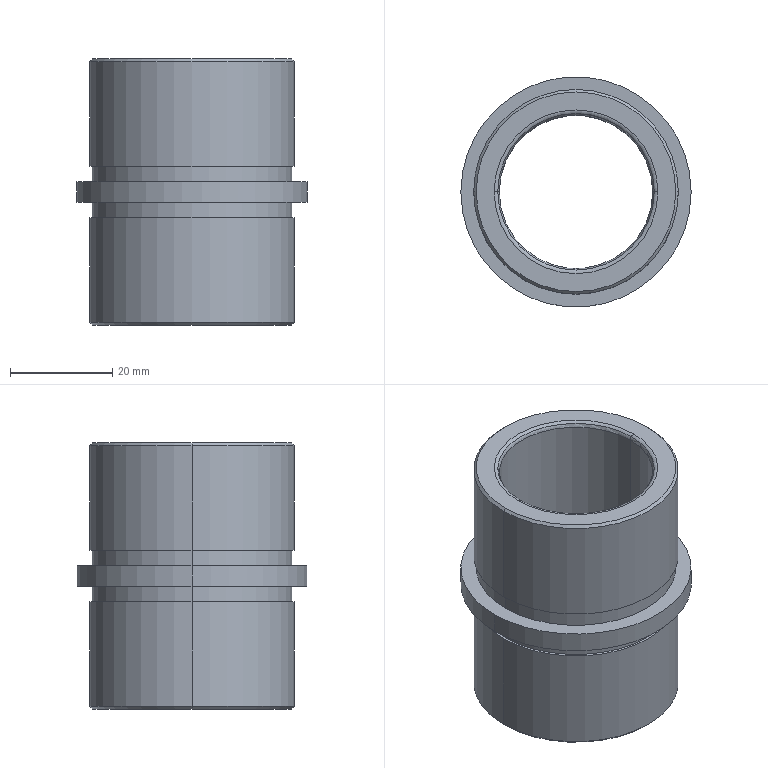Part | Creo | 1 solid | 30 faces | box 45 x 45 x 52 mm | volume 29479 mm3 | cylinder 12 | torus 8 | plane 6 | cone 4 | commonest cylinder face diameters 39 x4 40 x4 30 x2 45 x2
STEP:
#1=CARTESIAN_POINT('',(-187.5,-320.,-239.5));
#2=VERTEX_POINT('',#1);
#3=CARTESIAN_POINT('',(-142.5,-320.,-239.5));
#4=VERTEX_POINT('',#3);
#5=CARTESIAN_POINT('',(-165.,-320.,-239.5));
#6=DIRECTION('',(0.,0.,-1.));
#7=DIRECTION('',(-1.,0.,0.));
#8=AXIS2_PLACEMENT_3D('',#5,#6,#7);
#9=CIRCLE('',#8,22.5);
#10=EDGE_CURVE('',#2,#4,#9,.T.);
#11=ORIENTED_EDGE('',*,*,#10,.T.);
#12=CARTESIAN_POINT('',(-142.5,-320.,-235.5));
#13=VERTEX_POINT('',#12);
#14=CARTESIAN_POINT('',(-142.5,-320.,-239.5));
#15=DIRECTION('',(0.,0.,1.));
#16=VECTOR('',#15,4.);
#17=LINE('',#14,#16);
#18=EDGE_CURVE('',#4,#13,#17,.T.);
#19=ORIENTED_EDGE('',*,*,#18,.T.);
#20=CARTESIAN_POINT('',(-187.5,-320.,-235.5));
#21=VERTEX_POINT('',#20);
#22=CARTESIAN_POINT('',(-165.,-320.,-235.5));
#23=DIRECTION('',(0.,0.,1.));
#24=DIRECTION('',(1.,0.,0.));
#25=AXIS2_PLACEMENT_3D('',#22,#23,#24);
#26=CIRCLE('',#25,22.5);
#27=EDGE_CURVE('',#13,#21,#26,.T.);
#28=ORIENTED_EDGE('',*,*,#27,.T.);
#29=CARTESIAN_POINT('',(-187.5,-320.,-239.5));
#30=DIRECTION('',(0.,0.,1.));
#31=VECTOR('',#30,4.);
#32=LINE('',#29,#31);
#33=EDGE_CURVE('',#2,#21,#32,.T.);
#34=ORIENTED_EDGE('',*,*,#33,.F.);
#35=EDGE_LOOP('',(#11,#19,#28,#34));
#36=FACE_OUTER_BOUND('',#35,.F.);
#37=CARTESIAN_POINT('',(-165.,-320.,-239.5));
#38=DIRECTION('',(0.,0.,1.));
#39=DIRECTION('',(1.,0.,0.));
#40=AXIS2_PLACEMENT_3D('',#37,#38,#39);
#41=CYLINDRICAL_SURFACE('',#40,22.5);
#42=ADVANCED_FACE('',(#36),#41,.T.);
#43=CARTESIAN_POINT('',(-165.,-320.,-239.5));
#44=DIRECTION('',(0.,0.,-1.));
#45=DIRECTION('',(1.,0.,0.));
#46=AXIS2_PLACEMENT_3D('',#43,#44,#45);
#47=CIRCLE('',#46,22.5);
#48=EDGE_CURVE('',#4,#2,#47,.T.);
#49=ORIENTED_EDGE('',*,*,#48,.F.);
#50=ORIENTED_EDGE('',*,*,#10,.F.);
#51=EDGE_LOOP('',(#49,#50));
#52=FACE_OUTER_BOUND('',#51,.F.);
#53=CARTESIAN_POINT('',(-184.5,-320.,-239.5));
#54=VERTEX_POINT('',#53);
#55=CARTESIAN_POINT('',(-145.5,-320.,-239.5));
#56=VERTEX_POINT('',#55);
#57=CARTESIAN_POINT('',(-165.,-320.,-239.5));
#58=DIRECTION('',(0.,0.,1.));
#59=DIRECTION('',(-1.,0.,0.));
#60=AXIS2_PLACEMENT_3D('',#57,#58,#59);
#61=CIRCLE('',#60,19.5);
#62=EDGE_CURVE('',#54,#56,#61,.T.);
#63=ORIENTED_EDGE('',*,*,#62,.F.);
#64=CARTESIAN_POINT('',(-165.,-320.,-239.5));
#65=DIRECTION('',(0.,0.,1.));
#66=DIRECTION('',(1.,0.,0.));
#67=AXIS2_PLACEMENT_3D('',#64,#65,#66);
#68=CIRCLE('',#67,19.5);
#69=EDGE_CURVE('',#56,#54,#68,.T.);
#70=ORIENTED_EDGE('',*,*,#69,.F.);
#71=EDGE_LOOP('',(#63,#70));
#72=FACE_BOUND('',#71,.F.);
#73=CARTESIAN_POINT('',(-165.,-320.,-239.5));
#74=DIRECTION('',(0.,0.,1.));
#75=DIRECTION('',(1.,0.,0.));
#76=AXIS2_PLACEMENT_3D('',#73,#74,#75);
#77=PLANE('',#76);
#78=ADVANCED_FACE('',(#52,#72),#77,.F.);
#79=ORIENTED_EDGE('',*,*,#48,.T.);
#80=ORIENTED_EDGE('',*,*,#33,.T.);
#81=CARTESIAN_POINT('',(-165.,-320.,-235.5));
#82=DIRECTION('',(0.,0.,1.));
#83=DIRECTION('',(-1.,0.,0.));
#84=AXIS2_PLACEMENT_3D('',#81,#82,#83);
#85=CIRCLE('',#84,22.5);
#86=EDGE_CURVE('',#21,#13,#85,.T.);
#87=ORIENTED_EDGE('',*,*,#86,.T.);
#88=ORIENTED_EDGE('',*,*,#18,.F.);
#89=EDGE_LOOP('',(#79,#80,#87,#88));
#90=FACE_OUTER_BOUND('',#89,.F.);
#91=CARTESIAN_POINT('',(-165.,-320.,-239.5));
#92=DIRECTION('',(0.,0.,1.));
#93=DIRECTION('',(1.,0.,0.));
#94=AXIS2_PLACEMENT_3D('',#91,#92,#93);
#95=CYLINDRICAL_SURFACE('',#94,22.5);
#96=ADVANCED_FACE('',(#90),#95,.T.);
#97=ORIENTED_EDGE('',*,*,#27,.F.);
#98=ORIENTED_EDGE('',*,*,#86,.F.);
#99=EDGE_LOOP('',(#97,#98));
#100=FACE_OUTER_BOUND('',#99,.F.);
#101=CARTESIAN_POINT('',(-184.5,-320.,-235.5));
#102=VERTEX_POINT('',#101);
#103=CARTESIAN_POINT('',(-145.5,-320.,-235.5));
#104=VERTEX_POINT('',#103);
#105=CARTESIAN_POINT('',(-165.,-320.,-235.5));
#106=DIRECTION('',(0.,0.,-1.));
#107=DIRECTION('',(-1.,0.,0.));
#108=AXIS2_PLACEMENT_3D('',#105,#106,#107);
#109=CIRCLE('',#108,19.5);
#110=EDGE_CURVE('',#102,#104,#109,.T.);
#111=ORIENTED_EDGE('',*,*,#110,.F.);
#112=CARTESIAN_POINT('',(-165.,-320.,-235.5));
#113=DIRECTION('',(0.,0.,-1.));
#114=DIRECTION('',(1.,0.,0.));
#115=AXIS2_PLACEMENT_3D('',#112,#113,#114);
#116=CIRCLE('',#115,19.5);
#117=EDGE_CURVE('',#104,#102,#116,.T.);
#118=ORIENTED_EDGE('',*,*,#117,.F.);
#119=EDGE_LOOP('',(#111,#118));
#120=FACE_BOUND('',#119,.F.);
#121=CARTESIAN_POINT('',(-165.,-320.,-235.5));
#122=DIRECTION('',(0.,0.,1.));
#123=DIRECTION('',(1.,0.,0.));
#124=AXIS2_PLACEMENT_3D('',#121,#122,#123);
#125=PLANE('',#124);
#126=ADVANCED_FACE('',(#100,#120),#125,.T.);
#127=CARTESIAN_POINT('',(-145.5,-320.,-232.5));
#128=VERTEX_POINT('',#127);
#129=CARTESIAN_POINT('',(-184.5,-320.,-232.5));
#130=VERTEX_POINT('',#129);
#131=CARTESIAN_POINT('',(-165.,-320.,-232.5));
#132=DIRECTION('',(0.,0.,1.));
#133=DIRECTION('',(1.,0.,0.));
#134=AXIS2_PLACEMENT_3D('',#131,#132,#133);
#135=CIRCLE('',#134,19.5);
#136=EDGE_CURVE('',#128,#130,#135,.T.);
#137=ORIENTED_EDGE('',*,*,#136,.T.);
#138=CARTESIAN_POINT('',(-184.5,-320.,-232.5));
#139=DIRECTION('',(0.,0.,-1.));
#140=VECTOR('',#139,3.);
#141=LINE('',#138,#140);
#142=EDGE_CURVE('',#130,#102,#141,.T.);
#143=ORIENTED_EDGE('',*,*,#142,.T.);
#144=ORIENTED_EDGE('',*,*,#110,.T.);
#145=CARTESIAN_POINT('',(-145.5,-320.,-232.5));
#146=DIRECTION('',(0.,0.,-1.));
#147=VECTOR('',#146,3.);
#148=LINE('',#145,#147);
#149=EDGE_CURVE('',#128,#104,#148,.T.);
#150=ORIENTED_EDGE('',*,*,#149,.F.);
#151=EDGE_LOOP('',(#137,#143,#144,#150));
#152=FACE_OUTER_BOUND('',#151,.F.);
#153=CARTESIAN_POINT('',(-165.,-320.,-295.7));
#154=DIRECTION('',(0.,0.,-1.));
#155=DIRECTION('',(-1.,0.,0.));
#156=AXIS2_PLACEMENT_3D('',#153,#154,#155);
#157=CYLINDRICAL_SURFACE('',#156,19.5);
#158=ADVANCED_FACE('',(#152),#157,.T.);
#159=CARTESIAN_POINT('',(-145.,-320.,-232.5));
#160=VERTEX_POINT('',#159);
#161=CARTESIAN_POINT('',(-185.,-320.,-232.5));
#162=VERTEX_POINT('',#161);
#163=CARTESIAN_POINT('',(-165.,-320.,-232.5));
#164=DIRECTION('',(0.,0.,-1.));
#165=DIRECTION('',(1.,0.,0.));
#166=AXIS2_PLACEMENT_3D('',#163,#164,#165);
#167=CIRCLE('',#166,20.);
#168=EDGE_CURVE('',#160,#162,#167,.T.);
#169=ORIENTED_EDGE('',*,*,#168,.F.);
#170=CARTESIAN_POINT('',(-165.,-320.,-232.5));
#171=DIRECTION('',(0.,0.,-1.));
#172=DIRECTION('',(-1.,0.,0.));
#173=AXIS2_PLACEMENT_3D('',#170,#171,#172);
#174=CIRCLE('',#173,20.);
#175=EDGE_CURVE('',#162,#160,#174,.T.);
#176=ORIENTED_EDGE('',*,*,#175,.F.);
#177=EDGE_LOOP('',(#169,#176));
#178=FACE_OUTER_BOUND('',#177,.F.);
#179=CARTESIAN_POINT('',(-165.,-320.,-232.5));
#180=DIRECTION('',(0.,0.,1.));
#181=DIRECTION('',(-1.,0.,0.));
#182=AXIS2_PLACEMENT_3D('',#179,#180,#181);
#183=CIRCLE('',#182,19.5);
#184=EDGE_CURVE('',#130,#128,#183,.T.);
#185=ORIENTED_EDGE('',*,*,#184,.F.);
#186=ORIENTED_EDGE('',*,*,#136,.F.);
#187=EDGE_LOOP('',(#185,#186));
#188=FACE_BOUND('',#187,.F.);
#189=CARTESIAN_POINT('',(-110.,-320.,-232.5));
#190=DIRECTION('',(0.,0.,1.));
#191=DIRECTION('',(1.,0.,0.));
#192=AXIS2_PLACEMENT_3D('',#189,#190,#191);
#193=PLANE('',#192);
#194=ADVANCED_FACE('',(#178,#188),#193,.F.);
#195=CARTESIAN_POINT('',(-185.,-320.,-212.));
#196=VERTEX_POINT('',#195);
#197=CARTESIAN_POINT('',(-145.,-320.,-212.));
#198=VERTEX_POINT('',#197);
#199=CARTESIAN_POINT('',(-165.,-320.,-212.));
#200=DIRECTION('',(0.,0.,1.));
#201=DIRECTION('',(-1.,0.,0.));
#202=AXIS2_PLACEMENT_3D('',#199,#200,#201);
#203=CIRCLE('',#202,20.);
#204=EDGE_CURVE('',#196,#198,#203,.T.);
#205=ORIENTED_EDGE('',*,*,#204,.T.);
#206=CARTESIAN_POINT('',(-145.,-320.,-232.5));
#207=DIRECTION('',(0.,0.,1.));
#208=VECTOR('',#207,20.5);
#209=LINE('',#206,#208);
#210=EDGE_CURVE('',#160,#198,#209,.T.);
#211=ORIENTED_EDGE('',*,*,#210,.F.);
#212=ORIENTED_EDGE('',*,*,#168,.T.);
#213=CARTESIAN_POINT('',(-185.,-320.,-232.5));
#214=DIRECTION('',(0.,0.,1.));
#215=VECTOR('',#214,20.5);
#216=LINE('',#213,#215);
#217=EDGE_CURVE('',#162,#196,#216,.T.);
#218=ORIENTED_EDGE('',*,*,#217,.T.);
#219=EDGE_LOOP('',(#205,#211,#212,#218));
#220=FACE_OUTER_BOUND('',#219,.F.);
#221=CARTESIAN_POINT('',(-165.,-320.,-235.5));
#222=DIRECTION('',(0.,0.,1.));
#223=DIRECTION('',(1.,0.,0.));
#224=AXIS2_PLACEMENT_3D('',#221,#222,#223);
#225=CYLINDRICAL_SURFACE('',#224,20.);
#226=ADVANCED_FACE('',(#220),#225,.T.);
#227=ORIENTED_EDGE('',*,*,#204,.F.);
#228=CARTESIAN_POINT('',(-184.5,-320.,-211.5));
#229=VERTEX_POINT('',#228);
#230=CARTESIAN_POINT('',(-184.5,-320.,-211.5));
#231=DIRECTION('',(-0.7071,0.,-0.7071));
#232=VECTOR('',#231,0.7071);
#233=LINE('',#230,#232);
#234=EDGE_CURVE('',#229,#196,#233,.T.);
#235=ORIENTED_EDGE('',*,*,#234,.F.);
#236=CARTESIAN_POINT('',(-145.5,-320.,-211.5));
#237=VERTEX_POINT('',#236);
#238=CARTESIAN_POINT('',(-165.,-320.,-211.5));
#239=DIRECTION('',(0.,0.,1.));
#240=DIRECTION('',(-1.,0.,0.));
#241=AXIS2_PLACEMENT_3D('',#238,#239,#240);
#242=CIRCLE('',#241,19.5);
#243=EDGE_CURVE('',#229,#237,#242,.T.);
#244=ORIENTED_EDGE('',*,*,#243,.T.);
#245=CARTESIAN_POINT('',(-145.5,-320.,-211.5));
#246=DIRECTION('',(0.7071,0.,-0.7071));
#247=VECTOR('',#246,0.7071);
#248=LINE('',#245,#247);
#249=EDGE_CURVE('',#237,#198,#248,.T.);
#250=ORIENTED_EDGE('',*,*,#249,.T.);
#251=EDGE_LOOP('',(#227,#235,#244,#250));
#252=FACE_OUTER_BOUND('',#251,.F.);
#253=CARTESIAN_POINT('',(-165.,-320.,-211.75));
#254=DIRECTION('',(0.,0.,-1.));
#255=DIRECTION('',(-1.,0.,0.));
#256=AXIS2_PLACEMENT_3D('',#253,#254,#255);
#257=CONICAL_SURFACE('',#256,19.75,45.);
#258=ADVANCED_FACE('',(#252),#257,.T.);
#259=CARTESIAN_POINT('',(-165.,-320.,-212.));
#260=DIRECTION('',(0.,0.,1.));
#261=DIRECTION('',(1.,0.,0.));
#262=AXIS2_PLACEMENT_3D('',#259,#260,#261);
#263=CIRCLE('',#262,20.);
#264=EDGE_CURVE('',#198,#196,#263,.T.);
#265=ORIENTED_EDGE('',*,*,#264,.F.);
#266=ORIENTED_EDGE('',*,*,#249,.F.);
#267=CARTESIAN_POINT('',(-165.,-320.,-211.5));
#268=DIRECTION('',(0.,0.,1.));
#269=DIRECTION('',(1.,0.,0.));
#270=AXIS2_PLACEMENT_3D('',#267,#268,#269);
#271=CIRCLE('',#270,19.5);
#272=EDGE_CURVE('',#237,#229,#271,.T.);
#273=ORIENTED_EDGE('',*,*,#272,.T.);
#274=ORIENTED_EDGE('',*,*,#234,.T.);
#275=EDGE_LOOP('',(#265,#266,#273,#274));
#276=FACE_OUTER_BOUND('',#275,.F.);
#277=CARTESIAN_POINT('',(-165.,-320.,-211.75));
#278=DIRECTION('',(0.,0.,-1.));
#279=DIRECTION('',(-1.,0.,0.));
#280=AXIS2_PLACEMENT_3D('',#277,#278,#279);
#281=CONICAL_SURFACE('',#280,19.75,45.);
#282=ADVANCED_FACE('',(#276),#281,.T.);
#283=ORIENTED_EDGE('',*,*,#264,.T.);
#284=ORIENTED_EDGE('',*,*,#217,.F.);
#285=ORIENTED_EDGE('',*,*,#175,.T.);
#286=ORIENTED_EDGE('',*,*,#210,.T.);
#287=EDGE_LOOP('',(#283,#284,#285,#286));
#288=FACE_OUTER_BOUND('',#287,.F.);
#289=CARTESIAN_POINT('',(-165.,-320.,-235.5));
#290=DIRECTION('',(0.,0.,1.));
#291=DIRECTION('',(1.,0.,0.));
#292=AXIS2_PLACEMENT_3D('',#289,#290,#291);
#293=CYLINDRICAL_SURFACE('',#292,20.);
#294=ADVANCED_FACE('',(#288),#293,.T.);
#295=ORIENTED_EDGE('',*,*,#272,.F.);
#296=ORIENTED_EDGE('',*,*,#243,.F.);
#297=EDGE_LOOP('',(#295,#296));
#298=FACE_OUTER_BOUND('',#297,.F.);
#299=CARTESIAN_POINT('',(-149.,-320.,-211.5));
#300=VERTEX_POINT('',#299);
#301=CARTESIAN_POINT('',(-181.,-320.,-211.5));
#302=VERTEX_POINT('',#301);
#303=CARTESIAN_POINT('',(-165.,-320.,-211.5));
#304=DIRECTION('',(0.,0.,-1.));
#305=DIRECTION('',(1.,0.,0.));
#306=AXIS2_PLACEMENT_3D('',#303,#304,#305);
#307=CIRCLE('',#306,16.);
#308=EDGE_CURVE('',#300,#302,#307,.T.);
#309=ORIENTED_EDGE('',*,*,#308,.F.);
#310=CARTESIAN_POINT('',(-165.,-320.,-211.5));
#311=DIRECTION('',(0.,0.,-1.));
#312=DIRECTION('',(-1.,0.,0.));
#313=AXIS2_PLACEMENT_3D('',#310,#311,#312);
#314=CIRCLE('',#313,16.);
#315=EDGE_CURVE('',#302,#300,#314,.T.);
#316=ORIENTED_EDGE('',*,*,#315,.F.);
#317=EDGE_LOOP('',(#309,#316));
#318=FACE_BOUND('',#317,.F.);
#319=CARTESIAN_POINT('',(-165.,-320.,-211.5));
#320=DIRECTION('',(0.,0.,1.));
#321=DIRECTION('',(1.,0.,0.));
#322=AXIS2_PLACEMENT_3D('',#319,#320,#321);
#323=PLANE('',#322);
#324=ADVANCED_FACE('',(#298,#318),#323,.T.);
#325=ORIENTED_EDGE('',*,*,#308,.T.);
#326=CARTESIAN_POINT('',(-180.293,-320.,-211.793));
#327=VERTEX_POINT('',#326);
#328=CARTESIAN_POINT('',(-181.,-320.,-212.5));
#329=DIRECTION('',(0.,1.,0.));
#330=DIRECTION('',(0.,0.,1.));
#331=AXIS2_PLACEMENT_3D('',#328,#329,#330);
#332=CIRCLE('',#331,1.);
#333=EDGE_CURVE('',#302,#327,#332,.T.);
#334=ORIENTED_EDGE('',*,*,#333,.T.);
#335=CARTESIAN_POINT('',(-149.707,-320.,-211.793));
#336=VERTEX_POINT('',#335);
#337=CARTESIAN_POINT('',(-165.,-320.,-211.793));
#338=DIRECTION('',(0.,0.,1.));
#339=DIRECTION('',(-1.,0.,0.));
#340=AXIS2_PLACEMENT_3D('',#337,#338,#339);
#341=CIRCLE('',#340,15.293);
#342=EDGE_CURVE('',#327,#336,#341,.T.);
#343=ORIENTED_EDGE('',*,*,#342,.T.);
#344=CARTESIAN_POINT('',(-149.,-320.,-212.5));
#345=DIRECTION('',(0.,-1.,0.));
#346=DIRECTION('',(0.,0.,1.));
#347=AXIS2_PLACEMENT_3D('',#344,#345,#346);
#348=CIRCLE('',#347,1.);
#349=EDGE_CURVE('',#300,#336,#348,.T.);
#350=ORIENTED_EDGE('',*,*,#349,.F.);
#351=EDGE_LOOP('',(#325,#334,#343,#350));
#352=FACE_OUTER_BOUND('',#351,.F.);
#353=CARTESIAN_POINT('',(-165.,-320.,-212.5));
#354=DIRECTION('',(0.,0.,1.));
#355=DIRECTION('',(1.,0.,0.));
#356=AXIS2_PLACEMENT_3D('',#353,#354,#355);
#357=TOROIDAL_SURFACE('',#356,16.,1.);
#358=ADVANCED_FACE('',(#352),#357,.T.);
#359=ORIENTED_EDGE('',*,*,#315,.T.);
#360=ORIENTED_EDGE('',*,*,#349,.T.);
#361=CARTESIAN_POINT('',(-165.,-320.,-211.793));
#362=DIRECTION('',(0.,0.,1.));
#363=DIRECTION('',(1.,0.,0.));
#364=AXIS2_PLACEMENT_3D('',#361,#362,#363);
#365=CIRCLE('',#364,15.293);
#366=EDGE_CURVE('',#336,#327,#365,.T.);
#367=ORIENTED_EDGE('',*,*,#366,.T.);
#368=ORIENTED_EDGE('',*,*,#333,.F.);
#369=EDGE_LOOP('',(#359,#360,#367,#368));
#370=FACE_OUTER_BOUND('',#369,.F.);
#371=CARTESIAN_POINT('',(-165.,-320.,-212.5));
#372=DIRECTION('',(0.,0.,1.));
#373=DIRECTION('',(1.,0.,0.));
#374=AXIS2_PLACEMENT_3D('',#371,#372,#373);
#375=TOROIDAL_SURFACE('',#374,16.,1.);
#376=ADVANCED_FACE('',(#370),#375,.T.);
#377=CARTESIAN_POINT('',(-180.,-320.,-212.5));
#378=VERTEX_POINT('',#377);
#379=CARTESIAN_POINT('',(-150.,-320.,-212.5));
#380=VERTEX_POINT('',#379);
#381=CARTESIAN_POINT('',(-165.,-320.,-212.5));
#382=DIRECTION('',(0.,0.,-1.));
#383=DIRECTION('',(-1.,0.,0.));
#384=AXIS2_PLACEMENT_3D('',#381,#382,#383);
#385=CIRCLE('',#384,15.);
#386=EDGE_CURVE('',#378,#380,#385,.T.);
#387=ORIENTED_EDGE('',*,*,#386,.F.);
#388=CARTESIAN_POINT('',(-181.,-320.,-212.5));
#389=DIRECTION('',(0.,1.,0.));
#390=DIRECTION('',(0.7071,0.,0.7071));
#391=AXIS2_PLACEMENT_3D('',#388,#389,#390);
#392=CIRCLE('',#391,1.);
#393=EDGE_CURVE('',#327,#378,#392,.T.);
#394=ORIENTED_EDGE('',*,*,#393,.F.);
#395=ORIENTED_EDGE('',*,*,#366,.F.);
#396=CARTESIAN_POINT('',(-149.,-320.,-212.5));
#397=DIRECTION('',(0.,-1.,0.));
#398=DIRECTION('',(-0.7071,0.,0.7071));
#399=AXIS2_PLACEMENT_3D('',#396,#397,#398);
#400=CIRCLE('',#399,1.);
#401=EDGE_CURVE('',#336,#380,#400,.T.);
#402=ORIENTED_EDGE('',*,*,#401,.T.);
#403=EDGE_LOOP('',(#387,#394,#395,#402));
#404=FACE_OUTER_BOUND('',#403,.F.);
#405=CARTESIAN_POINT('',(-165.,-320.,-212.5));
#406=DIRECTION('',(0.,0.,1.));
#407=DIRECTION('',(1.,0.,0.));
#408=AXIS2_PLACEMENT_3D('',#405,#406,#407);
#409=TOROIDAL_SURFACE('',#408,16.,1.);
#410=ADVANCED_FACE('',(#404),#409,.T.);
#411=CARTESIAN_POINT('',(-150.,-320.,-262.5));
#412=VERTEX_POINT('',#411);
#413=CARTESIAN_POINT('',(-180.,-320.,-262.5));
#414=VERTEX_POINT('',#413);
#415=CARTESIAN_POINT('',(-165.,-320.,-262.5));
#416=DIRECTION('',(0.,0.,1.));
#417=DIRECTION('',(1.,0.,0.));
#418=AXIS2_PLACEMENT_3D('',#415,#416,#417);
#419=CIRCLE('',#418,15.);
#420=EDGE_CURVE('',#412,#414,#419,.T.);
#421=ORIENTED_EDGE('',*,*,#420,.T.);
#422=CARTESIAN_POINT('',(-180.,-320.,-212.5));
#423=DIRECTION('',(0.,0.,-1.));
#424=VECTOR('',#423,50.);
#425=LINE('',#422,#424);
#426=EDGE_CURVE('',#378,#414,#425,.T.);
#427=ORIENTED_EDGE('',*,*,#426,.F.);
#428=ORIENTED_EDGE('',*,*,#386,.T.);
#429=CARTESIAN_POINT('',(-150.,-320.,-212.5));
#430=DIRECTION('',(0.,0.,-1.));
#431=VECTOR('',#430,50.);
#432=LINE('',#429,#431);
#433=EDGE_CURVE('',#380,#412,#432,.T.);
#434=ORIENTED_EDGE('',*,*,#433,.T.);
#435=EDGE_LOOP('',(#421,#427,#428,#434));
#436=FACE_OUTER_BOUND('',#435,.F.);
#437=CARTESIAN_POINT('',(-165.,-320.,-211.5));
#438=DIRECTION('',(0.,0.,-1.));
#439=DIRECTION('',(-1.,0.,0.));
#440=AXIS2_PLACEMENT_3D('',#437,#438,#439);
#441=CYLINDRICAL_SURFACE('',#440,15.);
#442=ADVANCED_FACE('',(#436),#441,.F.);
#443=ORIENTED_EDGE('',*,*,#420,.F.);
#444=CARTESIAN_POINT('',(-149.707,-320.,-263.207));
#445=VERTEX_POINT('',#444);
#446=CARTESIAN_POINT('',(-149.,-320.,-262.5));
#447=DIRECTION('',(0.,1.,0.));
#448=DIRECTION('',(-0.7071,0.,-0.7071));
#449=AXIS2_PLACEMENT_3D('',#446,#447,#448);
#450=CIRCLE('',#449,1.);
#451=EDGE_CURVE('',#445,#412,#450,.T.);
#452=ORIENTED_EDGE('',*,*,#451,.F.);
#453=CARTESIAN_POINT('',(-180.293,-320.,-263.207));
#454=VERTEX_POINT('',#453);
#455=CARTESIAN_POINT('',(-165.,-320.,-263.207));
#456=DIRECTION('',(0.,0.,-1.));
#457=DIRECTION('',(-1.,0.,0.));
#458=AXIS2_PLACEMENT_3D('',#455,#456,#457);
#459=CIRCLE('',#458,15.293);
#460=EDGE_CURVE('',#454,#445,#459,.T.);
#461=ORIENTED_EDGE('',*,*,#460,.F.);
#462=CARTESIAN_POINT('',(-181.,-320.,-262.5));
#463=DIRECTION('',(0.,-1.,0.));
#464=DIRECTION('',(0.7071,0.,-0.7071));
#465=AXIS2_PLACEMENT_3D('',#462,#463,#464);
#466=CIRCLE('',#465,1.);
#467=EDGE_CURVE('',#454,#414,#466,.T.);
#468=ORIENTED_EDGE('',*,*,#467,.T.);
#469=EDGE_LOOP('',(#443,#452,#461,#468));
#470=FACE_OUTER_BOUND('',#469,.F.);
#471=CARTESIAN_POINT('',(-165.,-320.,-262.5));
#472=DIRECTION('',(0.,0.,-1.));
#473=DIRECTION('',(-1.,0.,0.));
#474=AXIS2_PLACEMENT_3D('',#471,#472,#473);
#475=TOROIDAL_SURFACE('',#474,16.,1.);
#476=ADVANCED_FACE('',(#470),#475,.T.);
#477=CARTESIAN_POINT('',(-165.,-320.,-262.5));
#478=DIRECTION('',(0.,0.,1.));
#479=DIRECTION('',(-1.,0.,0.));
#480=AXIS2_PLACEMENT_3D('',#477,#478,#479);
#481=CIRCLE('',#480,15.);
#482=EDGE_CURVE('',#414,#412,#481,.T.);
#483=ORIENTED_EDGE('',*,*,#482,.F.);
#484=ORIENTED_EDGE('',*,*,#467,.F.);
#485=CARTESIAN_POINT('',(-165.,-320.,-263.207));
#486=DIRECTION('',(0.,0.,-1.));
#487=DIRECTION('',(1.,0.,0.));
#488=AXIS2_PLACEMENT_3D('',#485,#486,#487);
#489=CIRCLE('',#488,15.293);
#490=EDGE_CURVE('',#445,#454,#489,.T.);
#491=ORIENTED_EDGE('',*,*,#490,.F.);
#492=ORIENTED_EDGE('',*,*,#451,.T.);
#493=EDGE_LOOP('',(#483,#484,#491,#492));
#494=FACE_OUTER_BOUND('',#493,.F.);
#495=CARTESIAN_POINT('',(-165.,-320.,-262.5));
#496=DIRECTION('',(0.,0.,-1.));
#497=DIRECTION('',(-1.,0.,0.));
#498=AXIS2_PLACEMENT_3D('',#495,#496,#497);
#499=TOROIDAL_SURFACE('',#498,16.,1.);
#500=ADVANCED_FACE('',(#494),#499,.T.);
#501=ORIENTED_EDGE('',*,*,#482,.T.);
#502=ORIENTED_EDGE('',*,*,#433,.F.);
#503=CARTESIAN_POINT('',(-165.,-320.,-212.5));
#504=DIRECTION('',(0.,0.,-1.));
#505=DIRECTION('',(1.,0.,0.));
#506=AXIS2_PLACEMENT_3D('',#503,#504,#505);
#507=CIRCLE('',#506,15.);
#508=EDGE_CURVE('',#380,#378,#507,.T.);
#509=ORIENTED_EDGE('',*,*,#508,.T.);
#510=ORIENTED_EDGE('',*,*,#426,.T.);
#511=EDGE_LOOP('',(#501,#502,#509,#510));
#512=FACE_OUTER_BOUND('',#511,.F.);
#513=CARTESIAN_POINT('',(-165.,-320.,-211.5));
#514=DIRECTION('',(0.,0.,-1.));
#515=DIRECTION('',(-1.,0.,0.));
#516=AXIS2_PLACEMENT_3D('',#513,#514,#515);
#517=CYLINDRICAL_SURFACE('',#516,15.);
#518=ADVANCED_FACE('',(#512),#517,.F.);
#519=ORIENTED_EDGE('',*,*,#508,.F.);
#520=ORIENTED_EDGE('',*,*,#401,.F.);
#521=ORIENTED_EDGE('',*,*,#342,.F.);
#522=ORIENTED_EDGE('',*,*,#393,.T.);
#523=EDGE_LOOP('',(#519,#520,#521,#522));
#524=FACE_OUTER_BOUND('',#523,.F.);
#525=CARTESIAN_POINT('',(-165.,-320.,-212.5));
#526=DIRECTION('',(0.,0.,1.));
#527=DIRECTION('',(1.,0.,0.));
#528=AXIS2_PLACEMENT_3D('',#525,#526,#527);
#529=TOROIDAL_SURFACE('',#528,16.,1.);
#530=ADVANCED_FACE('',(#524),#529,.T.);
#531=CARTESIAN_POINT('',(-181.,-320.,-263.5));
#532=VERTEX_POINT('',#531);
#533=CARTESIAN_POINT('',(-149.,-320.,-263.5));
#534=VERTEX_POINT('',#533);
#535=CARTESIAN_POINT('',(-165.,-320.,-263.5));
#536=DIRECTION('',(0.,0.,1.));
#537=DIRECTION('',(-1.,0.,0.));
#538=AXIS2_PLACEMENT_3D('',#535,#536,#537);
#539=CIRCLE('',#538,16.);
#540=EDGE_CURVE('',#532,#534,#539,.T.);
#541=ORIENTED_EDGE('',*,*,#540,.T.);
#542=CARTESIAN_POINT('',(-149.,-320.,-262.5));
#543=DIRECTION('',(0.,1.,0.));
#544=DIRECTION('',(0.,0.,-1.));
#545=AXIS2_PLACEMENT_3D('',#542,#543,#544);
#546=CIRCLE('',#545,1.);
#547=EDGE_CURVE('',#534,#445,#546,.T.);
#548=ORIENTED_EDGE('',*,*,#547,.T.);
#549=ORIENTED_EDGE('',*,*,#490,.T.);
#550=CARTESIAN_POINT('',(-181.,-320.,-262.5));
#551=DIRECTION('',(0.,-1.,0.));
#552=DIRECTION('',(0.,0.,-1.));
#553=AXIS2_PLACEMENT_3D('',#550,#551,#552);
#554=CIRCLE('',#553,1.);
#555=EDGE_CURVE('',#532,#454,#554,.T.);
#556=ORIENTED_EDGE('',*,*,#555,.F.);
#557=EDGE_LOOP('',(#541,#548,#549,#556));
#558=FACE_OUTER_BOUND('',#557,.F.);
#559=CARTESIAN_POINT('',(-165.,-320.,-262.5));
#560=DIRECTION('',(0.,0.,-1.));
#561=DIRECTION('',(-1.,0.,0.));
#562=AXIS2_PLACEMENT_3D('',#559,#560,#561);
#563=TOROIDAL_SURFACE('',#562,16.,1.);
#564=ADVANCED_FACE('',(#558),#563,.T.);
#565=CARTESIAN_POINT('',(-184.5,-320.,-263.5));
#566=VERTEX_POINT('',#565);
#567=CARTESIAN_POINT('',(-145.5,-320.,-263.5));
#568=VERTEX_POINT('',#567);
#569=CARTESIAN_POINT('',(-165.,-320.,-263.5));
#570=DIRECTION('',(0.,0.,-1.));
#571=DIRECTION('',(-1.,0.,0.));
#572=AXIS2_PLACEMENT_3D('',#569,#570,#571);
#573=CIRCLE('',#572,19.5);
#574=EDGE_CURVE('',#566,#568,#573,.T.);
#575=ORIENTED_EDGE('',*,*,#574,.F.);
#576=CARTESIAN_POINT('',(-165.,-320.,-263.5));
#577=DIRECTION('',(0.,0.,-1.));
#578=DIRECTION('',(1.,0.,0.));
#579=AXIS2_PLACEMENT_3D('',#576,#577,#578);
#580=CIRCLE('',#579,19.5);
#581=EDGE_CURVE('',#568,#566,#580,.T.);
#582=ORIENTED_EDGE('',*,*,#581,.F.);
#583=EDGE_LOOP('',(#575,#582));
#584=FACE_OUTER_BOUND('',#583,.F.);
#585=ORIENTED_EDGE('',*,*,#540,.F.);
#586=CARTESIAN_POINT('',(-165.,-320.,-263.5));
#587=DIRECTION('',(0.,0.,1.));
#588=DIRECTION('',(1.,0.,0.));
#589=AXIS2_PLACEMENT_3D('',#586,#587,#588);
#590=CIRCLE('',#589,16.);
#591=EDGE_CURVE('',#534,#532,#590,.T.);
#592=ORIENTED_EDGE('',*,*,#591,.F.);
#593=EDGE_LOOP('',(#585,#592));
#594=FACE_BOUND('',#593,.F.);
#595=CARTESIAN_POINT('',(-165.,-320.,-263.5));
#596=DIRECTION('',(0.,0.,-1.));
#597=DIRECTION('',(-1.,0.,0.));
#598=AXIS2_PLACEMENT_3D('',#595,#596,#597);
#599=PLANE('',#598);
#600=ADVANCED_FACE('',(#584,#594),#599,.T.);
#601=CARTESIAN_POINT('',(-185.,-320.,-263.));
#602=VERTEX_POINT('',#601);
#603=CARTESIAN_POINT('',(-145.,-320.,-263.));
#604=VERTEX_POINT('',#603);
#605=CARTESIAN_POINT('',(-165.,-320.,-263.));
#606=DIRECTION('',(0.,0.,-1.));
#607=DIRECTION('',(-1.,0.,0.));
#608=AXIS2_PLACEMENT_3D('',#605,#606,#607);
#609=CIRCLE('',#608,20.);
#610=EDGE_CURVE('',#602,#604,#609,.T.);
#611=ORIENTED_EDGE('',*,*,#610,.F.);
#612=CARTESIAN_POINT('',(-184.5,-320.,-263.5));
#613=DIRECTION('',(-0.7071,0.,0.7071));
#614=VECTOR('',#613,0.7071);
#615=LINE('',#612,#614);
#616=EDGE_CURVE('',#566,#602,#615,.T.);
#617=ORIENTED_EDGE('',*,*,#616,.F.);
#618=ORIENTED_EDGE('',*,*,#574,.T.);
#619=CARTESIAN_POINT('',(-145.5,-320.,-263.5));
#620=DIRECTION('',(0.7071,0.,0.7071));
#621=VECTOR('',#620,0.7071);
#622=LINE('',#619,#621);
#623=EDGE_CURVE('',#568,#604,#622,.T.);
#624=ORIENTED_EDGE('',*,*,#623,.T.);
#625=EDGE_LOOP('',(#611,#617,#618,#624));
#626=FACE_OUTER_BOUND('',#625,.F.);
#627=CARTESIAN_POINT('',(-165.,-320.,-263.25));
#628=DIRECTION('',(0.,0.,1.));
#629=DIRECTION('',(1.,0.,0.));
#630=AXIS2_PLACEMENT_3D('',#627,#628,#629);
#631=CONICAL_SURFACE('',#630,19.75,45.);
#632=ADVANCED_FACE('',(#626),#631,.T.);
#633=ORIENTED_EDGE('',*,*,#610,.T.);
#634=CARTESIAN_POINT('',(-145.,-320.,-242.5));
#635=VERTEX_POINT('',#634);
#636=CARTESIAN_POINT('',(-145.,-320.,-242.5));
#637=DIRECTION('',(0.,0.,-1.));
#638=VECTOR('',#637,20.5);
#639=LINE('',#636,#638);
#640=EDGE_CURVE('',#635,#604,#639,.T.);
#641=ORIENTED_EDGE('',*,*,#640,.F.);
#642=CARTESIAN_POINT('',(-185.,-320.,-242.5));
#643=VERTEX_POINT('',#642);
#644=CARTESIAN_POINT('',(-165.,-320.,-242.5));
#645=DIRECTION('',(0.,0.,1.));
#646=DIRECTION('',(1.,0.,0.));
#647=AXIS2_PLACEMENT_3D('',#644,#645,#646);
#648=CIRCLE('',#647,20.);
#649=EDGE_CURVE('',#635,#643,#648,.T.);
#650=ORIENTED_EDGE('',*,*,#649,.T.);
#651=CARTESIAN_POINT('',(-185.,-320.,-242.5));
#652=DIRECTION('',(0.,0.,-1.));
#653=VECTOR('',#652,20.5);
#654=LINE('',#651,#653);
#655=EDGE_CURVE('',#643,#602,#654,.T.);
#656=ORIENTED_EDGE('',*,*,#655,.T.);
#657=EDGE_LOOP('',(#633,#641,#650,#656));
#658=FACE_OUTER_BOUND('',#657,.F.);
#659=CARTESIAN_POINT('',(-165.,-320.,-239.5));
#660=DIRECTION('',(0.,0.,-1.));
#661=DIRECTION('',(-1.,0.,0.));
#662=AXIS2_PLACEMENT_3D('',#659,#660,#661);
#663=CYLINDRICAL_SURFACE('',#662,20.);
#664=ADVANCED_FACE('',(#658),#663,.T.);
#665=CARTESIAN_POINT('',(-165.,-320.,-263.));
#666=DIRECTION('',(0.,0.,-1.));
#667=DIRECTION('',(1.,0.,0.));
#668=AXIS2_PLACEMENT_3D('',#665,#666,#667);
#669=CIRCLE('',#668,20.);
#670=EDGE_CURVE('',#604,#602,#669,.T.);
#671=ORIENTED_EDGE('',*,*,#670,.T.);
#672=ORIENTED_EDGE('',*,*,#655,.F.);
#673=CARTESIAN_POINT('',(-165.,-320.,-242.5));
#674=DIRECTION('',(0.,0.,1.));
#675=DIRECTION('',(-1.,0.,0.));
#676=AXIS2_PLACEMENT_3D('',#673,#674,#675);
#677=CIRCLE('',#676,20.);
#678=EDGE_CURVE('',#643,#635,#677,.T.);
#679=ORIENTED_EDGE('',*,*,#678,.T.);
#680=ORIENTED_EDGE('',*,*,#640,.T.);
#681=EDGE_LOOP('',(#671,#672,#679,#680));
#682=FACE_OUTER_BOUND('',#681,.F.);
#683=CARTESIAN_POINT('',(-165.,-320.,-239.5));
#684=DIRECTION('',(0.,0.,-1.));
#685=DIRECTION('',(-1.,0.,0.));
#686=AXIS2_PLACEMENT_3D('',#683,#684,#685);
#687=CYLINDRICAL_SURFACE('',#686,20.);
#688=ADVANCED_FACE('',(#682),#687,.T.);
#689=ORIENTED_EDGE('',*,*,#670,.F.);
#690=ORIENTED_EDGE('',*,*,#623,.F.);
#691=ORIENTED_EDGE('',*,*,#581,.T.);
#692=ORIENTED_EDGE('',*,*,#616,.T.);
#693=EDGE_LOOP('',(#689,#690,#691,#692));
#694=FACE_OUTER_BOUND('',#693,.F.);
#695=CARTESIAN_POINT('',(-165.,-320.,-263.25));
#696=DIRECTION('',(0.,0.,1.));
#697=DIRECTION('',(1.,0.,0.));
#698=AXIS2_PLACEMENT_3D('',#695,#696,#697);
#699=CONICAL_SURFACE('',#698,19.75,45.);
#700=ADVANCED_FACE('',(#694),#699,.T.);
#701=ORIENTED_EDGE('',*,*,#678,.F.);
#702=ORIENTED_EDGE('',*,*,#649,.F.);
#703=EDGE_LOOP('',(#701,#702));
#704=FACE_OUTER_BOUND('',#703,.F.);
#705=CARTESIAN_POINT('',(-184.5,-320.,-242.5));
#706=VERTEX_POINT('',#705);
#707=CARTESIAN_POINT('',(-145.5,-320.,-242.5));
#708=VERTEX_POINT('',#707);
#709=CARTESIAN_POINT('',(-165.,-320.,-242.5));
#710=DIRECTION('',(0.,0.,-1.));
#711=DIRECTION('',(-1.,0.,0.));
#712=AXIS2_PLACEMENT_3D('',#709,#710,#711);
#713=CIRCLE('',#712,19.5);
#714=EDGE_CURVE('',#706,#708,#713,.T.);
#715=ORIENTED_EDGE('',*,*,#714,.F.);
#716=CARTESIAN_POINT('',(-165.,-320.,-242.5));
#717=DIRECTION('',(0.,0.,-1.));
#718=DIRECTION('',(1.,0.,0.));
#719=AXIS2_PLACEMENT_3D('',#716,#717,#718);
#720=CIRCLE('',#719,19.5);
#721=EDGE_CURVE('',#708,#706,#720,.T.);
#722=ORIENTED_EDGE('',*,*,#721,.F.);
#723=EDGE_LOOP('',(#715,#722));
#724=FACE_BOUND('',#723,.F.);
#725=CARTESIAN_POINT('',(-145.5,-320.,-242.5));
#726=DIRECTION('',(0.,0.,-1.));
#727=DIRECTION('',(-1.,0.,0.));
#728=AXIS2_PLACEMENT_3D('',#725,#726,#727);
#729=PLANE('',#728);
#730=ADVANCED_FACE('',(#704,#724),#729,.F.);
#731=ORIENTED_EDGE('',*,*,#69,.T.);
#732=CARTESIAN_POINT('',(-184.5,-320.,-239.5));
#733=DIRECTION('',(0.,0.,-1.));
#734=VECTOR('',#733,3.);
#735=LINE('',#732,#734);
#736=EDGE_CURVE('',#54,#706,#735,.T.);
#737=ORIENTED_EDGE('',*,*,#736,.T.);
#738=ORIENTED_EDGE('',*,*,#714,.T.);
#739=CARTESIAN_POINT('',(-145.5,-320.,-239.5));
#740=DIRECTION('',(0.,0.,-1.));
#741=VECTOR('',#740,3.);
#742=LINE('',#739,#741);
#743=EDGE_CURVE('',#56,#708,#742,.T.);
#744=ORIENTED_EDGE('',*,*,#743,.F.);
#745=EDGE_LOOP('',(#731,#737,#738,#744));
#746=FACE_OUTER_BOUND('',#745,.F.);
#747=CARTESIAN_POINT('',(-165.,-320.,-295.7));
#748=DIRECTION('',(0.,0.,-1.));
#749=DIRECTION('',(-1.,0.,0.));
#750=AXIS2_PLACEMENT_3D('',#747,#748,#749);
#751=CYLINDRICAL_SURFACE('',#750,19.5);
#752=ADVANCED_FACE('',(#746),#751,.T.);
#753=ORIENTED_EDGE('',*,*,#62,.T.);
#754=ORIENTED_EDGE('',*,*,#743,.T.);
#755=ORIENTED_EDGE('',*,*,#721,.T.);
#756=ORIENTED_EDGE('',*,*,#736,.F.);
#757=EDGE_LOOP('',(#753,#754,#755,#756));
#758=FACE_OUTER_BOUND('',#757,.F.);
#759=CARTESIAN_POINT('',(-165.,-320.,-295.7));
#760=DIRECTION('',(0.,0.,-1.));
#761=DIRECTION('',(-1.,0.,0.));
#762=AXIS2_PLACEMENT_3D('',#759,#760,#761);
#763=CYLINDRICAL_SURFACE('',#762,19.5);
#764=ADVANCED_FACE('',(#758),#763,.T.);
#765=ORIENTED_EDGE('',*,*,#591,.T.);
#766=ORIENTED_EDGE('',*,*,#555,.T.);
#767=ORIENTED_EDGE('',*,*,#460,.T.);
#768=ORIENTED_EDGE('',*,*,#547,.F.);
#769=EDGE_LOOP('',(#765,#766,#767,#768));
#770=FACE_OUTER_BOUND('',#769,.F.);
#771=CARTESIAN_POINT('',(-165.,-320.,-262.5));
#772=DIRECTION('',(0.,0.,-1.));
#773=DIRECTION('',(-1.,0.,0.));
#774=AXIS2_PLACEMENT_3D('',#771,#772,#773);
#775=TOROIDAL_SURFACE('',#774,16.,1.);
#776=ADVANCED_FACE('',(#770),#775,.T.);
#777=ORIENTED_EDGE('',*,*,#184,.T.);
#778=ORIENTED_EDGE('',*,*,#149,.T.);
#779=ORIENTED_EDGE('',*,*,#117,.T.);
#780=ORIENTED_EDGE('',*,*,#142,.F.);
#781=EDGE_LOOP('',(#777,#778,#779,#780));
#782=FACE_OUTER_BOUND('',#781,.F.);
#783=CARTESIAN_POINT('',(-165.,-320.,-295.7));
#784=DIRECTION('',(0.,0.,-1.));
#785=DIRECTION('',(-1.,0.,0.));
#786=AXIS2_PLACEMENT_3D('',#783,#784,#785);
#787=CYLINDRICAL_SURFACE('',#786,19.5);
#788=ADVANCED_FACE('',(#782),#787,.T.);
#789=CLOSED_SHELL('',(#42,#78,#96,#126,#158,#194,#226,#258,#282,#294,#324,#358,#376,#410,#442,#476,#500,#518,#530,#564,#600,#632,#664,#688,#700,#730,#752,#764,#776,#788));
#790=MANIFOLD_SOLID_BREP('',#789);
#791=(LENGTH_UNIT()NAMED_UNIT(*)SI_UNIT(.MILLI.,.METRE.));
#792=UNCERTAINTY_MEASURE_WITH_UNIT(LENGTH_MEASURE(0.008218),#791,'','');
#793=(NAMED_UNIT(*)PLANE_ANGLE_UNIT()SI_UNIT($,.RADIAN.));
#794=PLANE_ANGLE_MEASURE_WITH_UNIT(PLANE_ANGLE_MEASURE(0.01745),#793);
#795=(CONVERSION_BASED_UNIT('DEGREE',#794)NAMED_UNIT(*)PLANE_ANGLE_UNIT());
#796=(NAMED_UNIT(*)SI_UNIT($,.STERADIAN.)SOLID_ANGLE_UNIT());
#797=(GEOMETRIC_REPRESENTATION_CONTEXT(3)GLOBAL_UNCERTAINTY_ASSIGNED_CONTEXT((#792))GLOBAL_UNIT_ASSIGNED_CONTEXT((#791,#795,#796))REPRESENTATION_CONTEXT('',''));
#798=ADVANCED_BREP_SHAPE_REPRESENTATION('',(#790),#797);